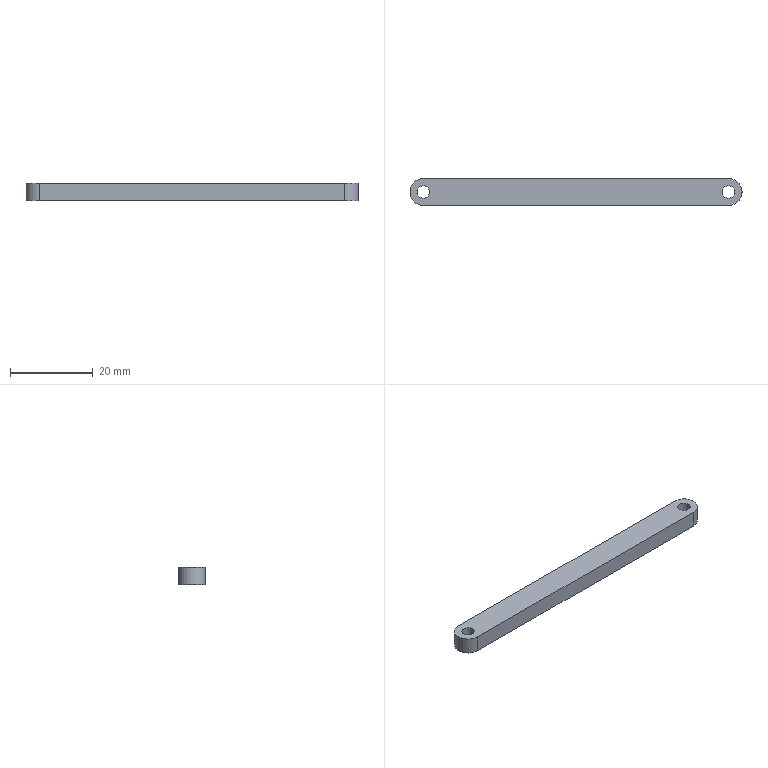Part | SolidWorks | features BaseBody 1 | 1 solid | 11 faces | box 80.131 x 6.513 x 4.119 mm | volume 2054 mm3 | cylinder 7 | plane 4 | commonest cylinder face diameters 3 x4 6.513 x3
STEP:
#1=CARTESIAN_POINT('',(294.529,516.78,0.));
#2=VERTEX_POINT('',#1);
#3=CARTESIAN_POINT('',(291.529,516.78,0.));
#4=VERTEX_POINT('',#3);
#5=CARTESIAN_POINT('',(293.029,516.78,0.));
#6=DIRECTION('',(0.,0.,-1.));
#7=DIRECTION('',(1.,0.,0.));
#8=AXIS2_PLACEMENT_3D('',#5,#6,#7);
#9=CIRCLE('',#8,1.5);
#10=EDGE_CURVE('',#2,#4,#9,.T.);
#11=ORIENTED_EDGE('',*,*,#10,.T.);
#12=CARTESIAN_POINT('',(291.529,516.78,4.119));
#13=VERTEX_POINT('',#12);
#14=CARTESIAN_POINT('',(291.529,516.78,0.));
#15=DIRECTION('',(0.,0.,1.));
#16=VECTOR('',#15,1000.);
#17=LINE('',#14,#16);
#18=EDGE_CURVE('',#4,#13,#17,.T.);
#19=ORIENTED_EDGE('',*,*,#18,.T.);
#20=CARTESIAN_POINT('',(294.529,516.78,4.119));
#21=VERTEX_POINT('',#20);
#22=CARTESIAN_POINT('',(293.029,516.78,4.119));
#23=DIRECTION('',(0.,0.,-1.));
#24=DIRECTION('',(1.,0.,0.));
#25=AXIS2_PLACEMENT_3D('',#22,#23,#24);
#26=CIRCLE('',#25,1.5);
#27=EDGE_CURVE('',#21,#13,#26,.T.);
#28=ORIENTED_EDGE('',*,*,#27,.F.);
#29=CARTESIAN_POINT('',(294.529,516.78,0.));
#30=DIRECTION('',(0.,0.,1.));
#31=VECTOR('',#30,1000.);
#32=LINE('',#29,#31);
#33=EDGE_CURVE('',#2,#21,#32,.T.);
#34=ORIENTED_EDGE('',*,*,#33,.F.);
#35=EDGE_LOOP('',(#11,#19,#28,#34));
#36=FACE_OUTER_BOUND('',#35,.T.);
#37=CARTESIAN_POINT('',(293.029,516.78,0.));
#38=DIRECTION('',(0.,0.,1.));
#39=DIRECTION('',(1.,0.,0.));
#40=AXIS2_PLACEMENT_3D('',#37,#38,#39);
#41=CYLINDRICAL_SURFACE('',#40,1.5);
#42=ADVANCED_FACE('',(#36),#41,.F.);
#43=CARTESIAN_POINT('',(220.911,516.78,0.));
#44=VERTEX_POINT('',#43);
#45=CARTESIAN_POINT('',(217.911,516.78,0.));
#46=VERTEX_POINT('',#45);
#47=CARTESIAN_POINT('',(219.411,516.78,0.));
#48=DIRECTION('',(0.,0.,-1.));
#49=DIRECTION('',(1.,0.,0.));
#50=AXIS2_PLACEMENT_3D('',#47,#48,#49);
#51=CIRCLE('',#50,1.5);
#52=EDGE_CURVE('',#44,#46,#51,.T.);
#53=ORIENTED_EDGE('',*,*,#52,.T.);
#54=CARTESIAN_POINT('',(217.911,516.78,4.119));
#55=VERTEX_POINT('',#54);
#56=CARTESIAN_POINT('',(217.911,516.78,0.));
#57=DIRECTION('',(0.,0.,1.));
#58=VECTOR('',#57,1000.);
#59=LINE('',#56,#58);
#60=EDGE_CURVE('',#46,#55,#59,.T.);
#61=ORIENTED_EDGE('',*,*,#60,.T.);
#62=CARTESIAN_POINT('',(220.911,516.78,4.119));
#63=VERTEX_POINT('',#62);
#64=CARTESIAN_POINT('',(219.411,516.78,4.119));
#65=DIRECTION('',(0.,0.,-1.));
#66=DIRECTION('',(1.,0.,0.));
#67=AXIS2_PLACEMENT_3D('',#64,#65,#66);
#68=CIRCLE('',#67,1.5);
#69=EDGE_CURVE('',#63,#55,#68,.T.);
#70=ORIENTED_EDGE('',*,*,#69,.F.);
#71=CARTESIAN_POINT('',(220.911,516.78,0.));
#72=DIRECTION('',(0.,0.,1.));
#73=VECTOR('',#72,1000.);
#74=LINE('',#71,#73);
#75=EDGE_CURVE('',#44,#63,#74,.T.);
#76=ORIENTED_EDGE('',*,*,#75,.F.);
#77=EDGE_LOOP('',(#53,#61,#70,#76));
#78=FACE_OUTER_BOUND('',#77,.T.);
#79=CARTESIAN_POINT('',(219.411,516.78,0.));
#80=DIRECTION('',(0.,0.,1.));
#81=DIRECTION('',(1.,0.,0.));
#82=AXIS2_PLACEMENT_3D('',#79,#80,#81);
#83=CYLINDRICAL_SURFACE('',#82,1.5);
#84=ADVANCED_FACE('',(#78),#83,.F.);
#85=CARTESIAN_POINT('',(293.029,513.523,0.));
#86=VERTEX_POINT('',#85);
#87=CARTESIAN_POINT('',(296.285,516.78,0.));
#88=VERTEX_POINT('',#87);
#89=CARTESIAN_POINT('',(293.029,516.78,0.));
#90=DIRECTION('',(0.,0.,1.));
#91=DIRECTION('',(1.,0.,0.));
#92=AXIS2_PLACEMENT_3D('',#89,#90,#91);
#93=CIRCLE('',#92,3.257);
#94=EDGE_CURVE('',#86,#88,#93,.T.);
#95=ORIENTED_EDGE('',*,*,#94,.T.);
#96=CARTESIAN_POINT('',(296.285,516.78,4.119));
#97=VERTEX_POINT('',#96);
#98=CARTESIAN_POINT('',(296.285,516.78,0.));
#99=DIRECTION('',(0.,0.,1.));
#100=VECTOR('',#99,1000.);
#101=LINE('',#98,#100);
#102=EDGE_CURVE('',#88,#97,#101,.T.);
#103=ORIENTED_EDGE('',*,*,#102,.T.);
#104=CARTESIAN_POINT('',(293.029,513.523,4.119));
#105=VERTEX_POINT('',#104);
#106=CARTESIAN_POINT('',(293.029,516.78,4.119));
#107=DIRECTION('',(0.,0.,-1.));
#108=DIRECTION('',(1.,0.,0.));
#109=AXIS2_PLACEMENT_3D('',#106,#107,#108);
#110=CIRCLE('',#109,3.257);
#111=EDGE_CURVE('',#97,#105,#110,.T.);
#112=ORIENTED_EDGE('',*,*,#111,.T.);
#113=CARTESIAN_POINT('',(293.029,513.523,0.));
#114=DIRECTION('',(0.,0.,-1.));
#115=VECTOR('',#114,1000.);
#116=LINE('',#113,#115);
#117=EDGE_CURVE('',#105,#86,#116,.T.);
#118=ORIENTED_EDGE('',*,*,#117,.T.);
#119=EDGE_LOOP('',(#95,#103,#112,#118));
#120=FACE_OUTER_BOUND('',#119,.T.);
#121=CARTESIAN_POINT('',(293.029,516.78,0.));
#122=DIRECTION('',(0.,0.,1.));
#123=DIRECTION('',(1.,0.,0.));
#124=AXIS2_PLACEMENT_3D('',#121,#122,#123);
#125=CYLINDRICAL_SURFACE('',#124,3.257);
#126=ADVANCED_FACE('',(#120),#125,.T.);
#127=ORIENTED_EDGE('',*,*,#10,.F.);
#128=CARTESIAN_POINT('',(293.029,516.78,0.));
#129=DIRECTION('',(0.,0.,-1.));
#130=DIRECTION('',(1.,0.,0.));
#131=AXIS2_PLACEMENT_3D('',#128,#129,#130);
#132=CIRCLE('',#131,1.5);
#133=EDGE_CURVE('',#4,#2,#132,.T.);
#134=ORIENTED_EDGE('',*,*,#133,.F.);
#135=EDGE_LOOP('',(#127,#134));
#136=FACE_BOUND('',#135,.T.);
#137=ORIENTED_EDGE('',*,*,#52,.F.);
#138=CARTESIAN_POINT('',(219.411,516.78,0.));
#139=DIRECTION('',(0.,0.,-1.));
#140=DIRECTION('',(1.,0.,0.));
#141=AXIS2_PLACEMENT_3D('',#138,#139,#140);
#142=CIRCLE('',#141,1.5);
#143=EDGE_CURVE('',#46,#44,#142,.T.);
#144=ORIENTED_EDGE('',*,*,#143,.F.);
#145=EDGE_LOOP('',(#137,#144));
#146=FACE_BOUND('',#145,.T.);
#147=ORIENTED_EDGE('',*,*,#94,.F.);
#148=CARTESIAN_POINT('',(219.411,513.523,0.));
#149=VERTEX_POINT('',#148);
#150=CARTESIAN_POINT('',(256.22,513.523,0.));
#151=DIRECTION('',(1.,0.,0.));
#152=VECTOR('',#151,1000.);
#153=LINE('',#150,#152);
#154=EDGE_CURVE('',#149,#86,#153,.T.);
#155=ORIENTED_EDGE('',*,*,#154,.F.);
#156=CARTESIAN_POINT('',(219.411,520.037,0.));
#157=VERTEX_POINT('',#156);
#158=CARTESIAN_POINT('',(219.411,516.78,0.));
#159=DIRECTION('',(0.,0.,1.));
#160=DIRECTION('',(1.,0.,0.));
#161=AXIS2_PLACEMENT_3D('',#158,#159,#160);
#162=CIRCLE('',#161,3.257);
#163=EDGE_CURVE('',#157,#149,#162,.T.);
#164=ORIENTED_EDGE('',*,*,#163,.F.);
#165=CARTESIAN_POINT('',(293.029,520.037,0.));
#166=VERTEX_POINT('',#165);
#167=CARTESIAN_POINT('',(256.22,520.037,0.));
#168=DIRECTION('',(-1.,0.,0.));
#169=VECTOR('',#168,1000.);
#170=LINE('',#167,#169);
#171=EDGE_CURVE('',#166,#157,#170,.T.);
#172=ORIENTED_EDGE('',*,*,#171,.F.);
#173=CARTESIAN_POINT('',(293.029,516.78,0.));
#174=DIRECTION('',(0.,0.,1.));
#175=DIRECTION('',(1.,0.,0.));
#176=AXIS2_PLACEMENT_3D('',#173,#174,#175);
#177=CIRCLE('',#176,3.257);
#178=EDGE_CURVE('',#88,#166,#177,.T.);
#179=ORIENTED_EDGE('',*,*,#178,.F.);
#180=EDGE_LOOP('',(#147,#155,#164,#172,#179));
#181=FACE_OUTER_BOUND('',#180,.T.);
#182=CARTESIAN_POINT('',(256.22,516.78,0.));
#183=DIRECTION('',(0.,0.,1.));
#184=DIRECTION('',(1.,0.,0.));
#185=AXIS2_PLACEMENT_3D('',#182,#183,#184);
#186=PLANE('',#185);
#187=ADVANCED_FACE('',(#136,#146,#181),#186,.F.);
#188=ORIENTED_EDGE('',*,*,#18,.F.);
#189=ORIENTED_EDGE('',*,*,#133,.T.);
#190=ORIENTED_EDGE('',*,*,#33,.T.);
#191=CARTESIAN_POINT('',(293.029,516.78,4.119));
#192=DIRECTION('',(0.,0.,-1.));
#193=DIRECTION('',(1.,0.,0.));
#194=AXIS2_PLACEMENT_3D('',#191,#192,#193);
#195=CIRCLE('',#194,1.5);
#196=EDGE_CURVE('',#13,#21,#195,.T.);
#197=ORIENTED_EDGE('',*,*,#196,.F.);
#198=EDGE_LOOP('',(#188,#189,#190,#197));
#199=FACE_OUTER_BOUND('',#198,.T.);
#200=CARTESIAN_POINT('',(293.029,516.78,0.));
#201=DIRECTION('',(0.,0.,1.));
#202=DIRECTION('',(1.,0.,0.));
#203=AXIS2_PLACEMENT_3D('',#200,#201,#202);
#204=CYLINDRICAL_SURFACE('',#203,1.5);
#205=ADVANCED_FACE('',(#199),#204,.F.);
#206=ORIENTED_EDGE('',*,*,#60,.F.);
#207=ORIENTED_EDGE('',*,*,#143,.T.);
#208=ORIENTED_EDGE('',*,*,#75,.T.);
#209=CARTESIAN_POINT('',(219.411,516.78,4.119));
#210=DIRECTION('',(0.,0.,-1.));
#211=DIRECTION('',(1.,0.,0.));
#212=AXIS2_PLACEMENT_3D('',#209,#210,#211);
#213=CIRCLE('',#212,1.5);
#214=EDGE_CURVE('',#55,#63,#213,.T.);
#215=ORIENTED_EDGE('',*,*,#214,.F.);
#216=EDGE_LOOP('',(#206,#207,#208,#215));
#217=FACE_OUTER_BOUND('',#216,.T.);
#218=CARTESIAN_POINT('',(219.411,516.78,0.));
#219=DIRECTION('',(0.,0.,1.));
#220=DIRECTION('',(1.,0.,0.));
#221=AXIS2_PLACEMENT_3D('',#218,#219,#220);
#222=CYLINDRICAL_SURFACE('',#221,1.5);
#223=ADVANCED_FACE('',(#217),#222,.F.);
#224=ORIENTED_EDGE('',*,*,#171,.T.);
#225=CARTESIAN_POINT('',(219.411,520.037,4.119));
#226=VERTEX_POINT('',#225);
#227=CARTESIAN_POINT('',(219.411,520.037,0.));
#228=DIRECTION('',(0.,0.,1.));
#229=VECTOR('',#228,1000.);
#230=LINE('',#227,#229);
#231=EDGE_CURVE('',#157,#226,#230,.T.);
#232=ORIENTED_EDGE('',*,*,#231,.T.);
#233=CARTESIAN_POINT('',(293.029,520.037,4.119));
#234=VERTEX_POINT('',#233);
#235=CARTESIAN_POINT('',(293.029,520.037,4.119));
#236=DIRECTION('',(1.,0.,0.));
#237=VECTOR('',#236,1000.);
#238=LINE('',#235,#237);
#239=EDGE_CURVE('',#226,#234,#238,.T.);
#240=ORIENTED_EDGE('',*,*,#239,.T.);
#241=CARTESIAN_POINT('',(293.029,520.037,0.));
#242=DIRECTION('',(0.,0.,-1.));
#243=VECTOR('',#242,1000.);
#244=LINE('',#241,#243);
#245=EDGE_CURVE('',#234,#166,#244,.T.);
#246=ORIENTED_EDGE('',*,*,#245,.T.);
#247=EDGE_LOOP('',(#224,#232,#240,#246));
#248=FACE_OUTER_BOUND('',#247,.T.);
#249=CARTESIAN_POINT('',(293.029,520.037,0.));
#250=DIRECTION('',(0.,1.,0.));
#251=DIRECTION('',(0.,0.,1.));
#252=AXIS2_PLACEMENT_3D('',#249,#250,#251);
#253=PLANE('',#252);
#254=ADVANCED_FACE('',(#248),#253,.T.);
#255=ORIENTED_EDGE('',*,*,#102,.F.);
#256=ORIENTED_EDGE('',*,*,#178,.T.);
#257=ORIENTED_EDGE('',*,*,#245,.F.);
#258=CARTESIAN_POINT('',(293.029,516.78,4.119));
#259=DIRECTION('',(0.,0.,-1.));
#260=DIRECTION('',(1.,0.,0.));
#261=AXIS2_PLACEMENT_3D('',#258,#259,#260);
#262=CIRCLE('',#261,3.257);
#263=EDGE_CURVE('',#234,#97,#262,.T.);
#264=ORIENTED_EDGE('',*,*,#263,.T.);
#265=EDGE_LOOP('',(#255,#256,#257,#264));
#266=FACE_OUTER_BOUND('',#265,.T.);
#267=CARTESIAN_POINT('',(293.029,516.78,0.));
#268=DIRECTION('',(0.,0.,1.));
#269=DIRECTION('',(1.,0.,0.));
#270=AXIS2_PLACEMENT_3D('',#267,#268,#269);
#271=CYLINDRICAL_SURFACE('',#270,3.257);
#272=ADVANCED_FACE('',(#266),#271,.T.);
#273=ORIENTED_EDGE('',*,*,#154,.T.);
#274=ORIENTED_EDGE('',*,*,#117,.F.);
#275=CARTESIAN_POINT('',(219.411,513.523,4.119));
#276=VERTEX_POINT('',#275);
#277=CARTESIAN_POINT('',(219.411,513.523,4.119));
#278=DIRECTION('',(-1.,0.,0.));
#279=VECTOR('',#278,1000.);
#280=LINE('',#277,#279);
#281=EDGE_CURVE('',#105,#276,#280,.T.);
#282=ORIENTED_EDGE('',*,*,#281,.T.);
#283=CARTESIAN_POINT('',(219.411,513.523,0.));
#284=DIRECTION('',(0.,0.,-1.));
#285=VECTOR('',#284,1000.);
#286=LINE('',#283,#285);
#287=EDGE_CURVE('',#276,#149,#286,.T.);
#288=ORIENTED_EDGE('',*,*,#287,.T.);
#289=EDGE_LOOP('',(#273,#274,#282,#288));
#290=FACE_OUTER_BOUND('',#289,.T.);
#291=CARTESIAN_POINT('',(219.411,513.523,0.));
#292=DIRECTION('',(0.,-1.,0.));
#293=DIRECTION('',(0.,0.,-1.));
#294=AXIS2_PLACEMENT_3D('',#291,#292,#293);
#295=PLANE('',#294);
#296=ADVANCED_FACE('',(#290),#295,.T.);
#297=ORIENTED_EDGE('',*,*,#163,.T.);
#298=ORIENTED_EDGE('',*,*,#287,.F.);
#299=CARTESIAN_POINT('',(219.411,516.78,4.119));
#300=DIRECTION('',(0.,0.,-1.));
#301=DIRECTION('',(1.,0.,0.));
#302=AXIS2_PLACEMENT_3D('',#299,#300,#301);
#303=CIRCLE('',#302,3.257);
#304=EDGE_CURVE('',#276,#226,#303,.T.);
#305=ORIENTED_EDGE('',*,*,#304,.T.);
#306=ORIENTED_EDGE('',*,*,#231,.F.);
#307=EDGE_LOOP('',(#297,#298,#305,#306));
#308=FACE_OUTER_BOUND('',#307,.T.);
#309=CARTESIAN_POINT('',(219.411,516.78,0.));
#310=DIRECTION('',(0.,0.,1.));
#311=DIRECTION('',(1.,0.,0.));
#312=AXIS2_PLACEMENT_3D('',#309,#310,#311);
#313=CYLINDRICAL_SURFACE('',#312,3.257);
#314=ADVANCED_FACE('',(#308),#313,.T.);
#315=ORIENTED_EDGE('',*,*,#27,.T.);
#316=ORIENTED_EDGE('',*,*,#196,.T.);
#317=EDGE_LOOP('',(#315,#316));
#318=FACE_BOUND('',#317,.T.);
#319=ORIENTED_EDGE('',*,*,#69,.T.);
#320=ORIENTED_EDGE('',*,*,#214,.T.);
#321=EDGE_LOOP('',(#319,#320));
#322=FACE_BOUND('',#321,.T.);
#323=ORIENTED_EDGE('',*,*,#239,.F.);
#324=ORIENTED_EDGE('',*,*,#304,.F.);
#325=ORIENTED_EDGE('',*,*,#281,.F.);
#326=ORIENTED_EDGE('',*,*,#111,.F.);
#327=ORIENTED_EDGE('',*,*,#263,.F.);
#328=EDGE_LOOP('',(#323,#324,#325,#326,#327));
#329=FACE_OUTER_BOUND('',#328,.T.);
#330=CARTESIAN_POINT('',(256.22,516.78,4.119));
#331=DIRECTION('',(0.,0.,-1.));
#332=DIRECTION('',(-1.,0.,0.));
#333=AXIS2_PLACEMENT_3D('',#330,#331,#332);
#334=PLANE('',#333);
#335=ADVANCED_FACE('',(#318,#322,#329),#334,.F.);
#336=CLOSED_SHELL('',(#42,#84,#126,#187,#205,#223,#254,#272,#296,#314,#335));
#337=MANIFOLD_SOLID_BREP('',#336);
#338=CARTESIAN_POINT('',(0.,0.,0.));
#339=DIRECTION('',(0.,0.,1.));
#340=DIRECTION('',(1.,0.,0.));
#341=AXIS2_PLACEMENT_3D('',#338,#339,#340);
#342=(LENGTH_UNIT()NAMED_UNIT(*)SI_UNIT(.MILLI.,.METRE.));
#343=UNCERTAINTY_MEASURE_WITH_UNIT(LENGTH_MEASURE(0.00001),#342,'','');
#344=(NAMED_UNIT(*)PLANE_ANGLE_UNIT()SI_UNIT($,.RADIAN.));
#345=(NAMED_UNIT(*)SI_UNIT($,.STERADIAN.)SOLID_ANGLE_UNIT());
#346=(GEOMETRIC_REPRESENTATION_CONTEXT(3)GLOBAL_UNCERTAINTY_ASSIGNED_CONTEXT((#343))GLOBAL_UNIT_ASSIGNED_CONTEXT((#342,#344,#345))REPRESENTATION_CONTEXT('',''));
#347=ADVANCED_BREP_SHAPE_REPRESENTATION('',(#337,#341),#346);